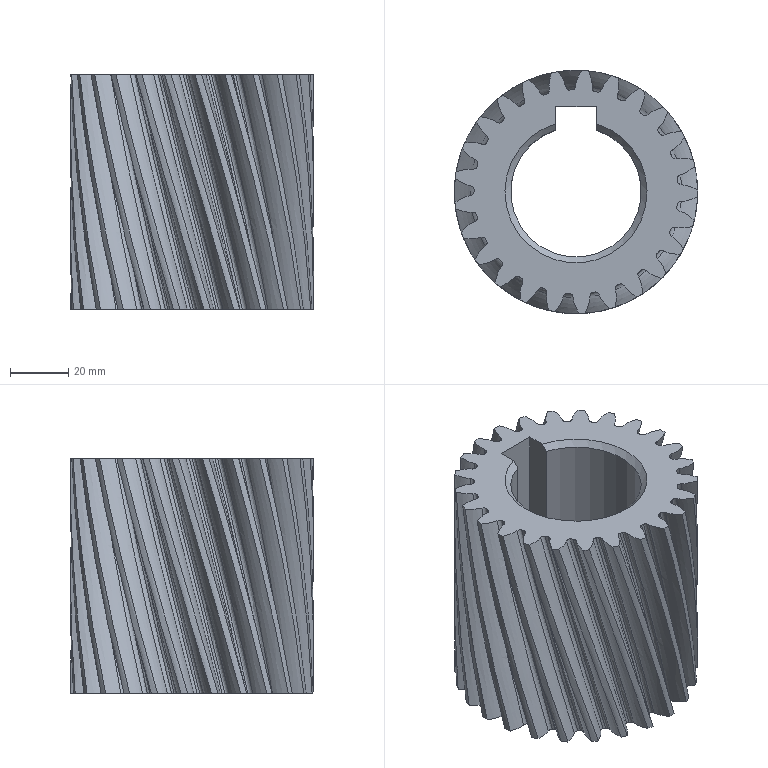Part | NX | 1 solid | 158 faces | box 83.83 x 83.83 x 81 mm | volume 243039 mm3 | spline 125 | cylinder 26 | plane 5 | cone 2 | commonest cylinder face diameters 70.33 x25 45 x1